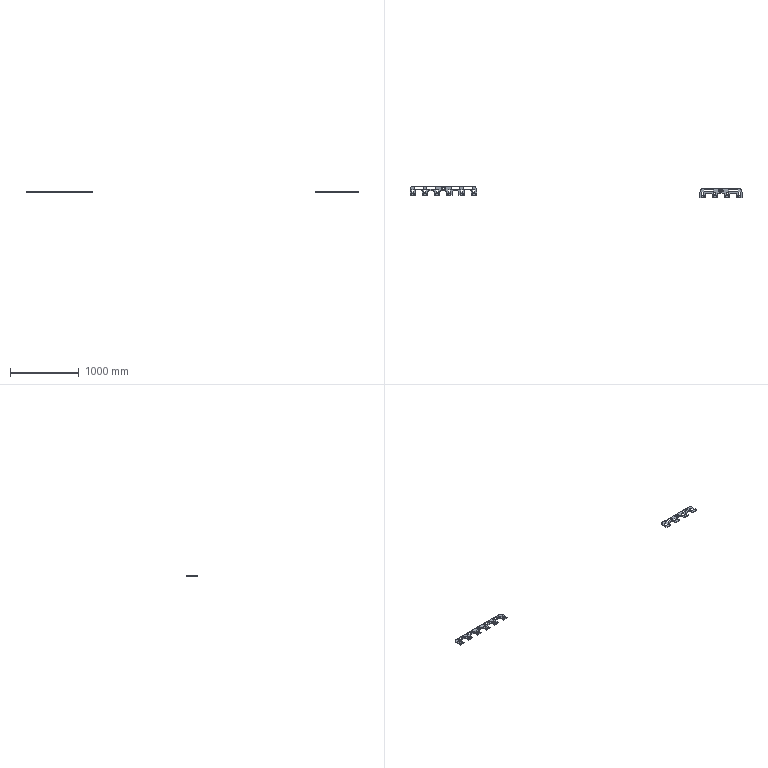NC program | NX | posted with a generic post | part box 4825 x 168.213 x 13 mm
Lines 124 to 1113 of 9095:
(ZLEVEL_PROFILE , TOOL : D10)
N228 T10 M6
N230 G54
N232 G17 G0 G90 X-46.824 Y72.1 S9500 M3
N234 G43 Z30. H10
N236 Z1.5
N238 G94 G1 X-0.002 Z-0.954 F1000.
N240 X255.6 F3500.
N242 G2 X310.7 Y16.999 R55.1
N244 G1 Y-67.
N246 G2 X305.6 Y-72.1 R5.1
N248 G1 X227.8
N250 G2 X222.7 Y-67. R5.1
N252 G1 Y-20.95
N254 G3 X207.8 Y-6.05 R14.9
N256 G1 X147.8
N258 G3 X132.9 Y-20.95 R14.9
N260 G1 Y-67.
N262 G2 X127.8 Y-72.1 R5.1
N264 G1 X50.
N266 G2 X44.9 Y-67. R5.1
N268 G1 Y-20.95
N270 G3 X30. Y-6.05 R14.9
N272 G1 X-30.
N274 G3 X-44.9 Y-20.95 R14.9
N276 G1 Y-67.
N278 G2 X-50. Y-72.1 R5.1
N280 G1 X-127.8
N282 G2 X-132.9 Y-67. R5.1
N284 G1 Y-20.95
N286 G3 X-147.8 Y-6.05 R14.9
N288 G1 X-207.804
N290 G3 X-222.7 Y-20.95 R14.9
N292 G1 Y-67.
N294 G2 X-227.8 Y-72.1 R5.1
N296 G1 X-305.6
N298 G2 X-310.7 Y-67. R5.1
N300 G1 Y16.999
N302 G2 X-255.604 Y72.1 R55.1
N304 G1 X-0.002
N306 X54.644 Z-1.908
N308 X255.6
N310 G2 X310.7 Y16.999 R55.1
N312 G1 Y-67.
N314 G2 X305.6 Y-72.1 R5.1
N316 G1 X227.8
N318 G2 X222.7 Y-67. R5.1
N320 G1 Y-20.95
N322 G3 X207.8 Y-6.05 R14.9
N324 G1 X147.8
N326 G3 X132.9 Y-20.95 R14.9
N328 G1 Y-67.
N330 G2 X127.8 Y-72.1 R5.1
N332 G1 X50.
N334 G2 X44.9 Y-67. R5.1
N336 G1 Y-20.95
N338 G3 X30. Y-6.05 R14.9
N340 G1 X-30.
N342 G3 X-44.9 Y-20.95 R14.9
N344 G1 Y-67.
N346 G2 X-50. Y-72.1 R5.1
N348 G1 X-127.8
N350 G2 X-132.9 Y-67. R5.1
N352 G1 Y-20.95
N354 G3 X-147.8 Y-6.05 R14.9
N356 G1 X-207.804
N358 G3 X-222.7 Y-20.95 R14.9
N360 G1 Y-67.
N362 G2 X-227.8 Y-72.1 R5.1
N364 G1 X-305.6
N366 G2 X-310.7 Y-67. R5.1
N368 G1 Y16.999
N370 G2 X-255.604 Y72.1 R55.1
N372 G1 X-0.002
N374 X54.644 Z-2.862
N376 X255.6
N378 G2 X310.7 Y16.999 R55.1
N380 G1 Y-67.
N382 G2 X305.6 Y-72.1 R5.1
N384 G1 X227.8
N386 G2 X222.7 Y-67. R5.1
N388 G1 Y-20.95
N390 G3 X207.8 Y-6.05 R14.9
N392 G1 X147.8
N394 G3 X132.9 Y-20.95 R14.9
N396 G1 Y-67.
N398 G2 X127.8 Y-72.1 R5.1
N400 G1 X50.
N402 G2 X44.9 Y-67. R5.1
N404 G1 Y-20.95
N406 G3 X30. Y-6.05 R14.9
N408 G1 X-30.
N410 G3 X-44.9 Y-20.95 R14.9
N412 G1 Y-67.
N414 G2 X-50. Y-72.1 R5.1
N416 G1 X-127.8
N418 G2 X-132.9 Y-67. R5.1
N420 G1 Y-20.95
N422 G3 X-147.8 Y-6.05 R14.9
N424 G1 X-207.804
N426 G3 X-222.7 Y-20.95 R14.9
N428 G1 Y-67.
N430 G2 X-227.8 Y-72.1 R5.1
N432 G1 X-305.6
N434 G2 X-310.7 Y-67. R5.1
N436 G1 Y16.999
N438 G2 X-255.604 Y72.1 R55.1
N440 G1 X-0.002
N442 X54.644 Z-3.815
N444 X255.6
N446 G2 X310.7 Y16.999 R55.1
N448 G1 Y-67.
N450 G2 X305.6 Y-72.1 R5.1
N452 G1 X227.8
N454 G2 X222.7 Y-67. R5.1
N456 G1 Y-20.95
N458 G3 X207.8 Y-6.05 R14.9
N460 G1 X147.8
N462 G3 X132.9 Y-20.95 R14.9
N464 G1 Y-67.
N466 G2 X127.8 Y-72.1 R5.1
N468 G1 X50.
N470 G2 X44.9 Y-67. R5.1
N472 G1 Y-20.95
N474 G3 X30. Y-6.05 R14.9
N476 G1 X-30.
N478 G3 X-44.9 Y-20.95 R14.9
N480 G1 Y-67.
N482 G2 X-50. Y-72.1 R5.1
N484 G1 X-127.8
N486 G2 X-132.9 Y-67. R5.1
N488 G1 Y-20.95
N490 G3 X-147.8 Y-6.05 R14.9
N492 G1 X-207.804
N494 G3 X-222.7 Y-20.95 R14.9
N496 G1 Y-67.
N498 G2 X-227.8 Y-72.1 R5.1
N500 G1 X-305.6
N502 G2 X-310.7 Y-67. R5.1
N504 G1 Y16.999
N506 G2 X-255.604 Y72.1 R55.1
N508 G1 X-0.002
N510 X54.644 Z-4.769
N512 X255.6
N514 G2 X310.7 Y16.999 R55.1
N516 G1 Y-67.
N518 G2 X305.6 Y-72.1 R5.1
N520 G1 X227.8
N522 G2 X222.7 Y-67. R5.1
N524 G1 Y-20.95
N526 G3 X207.8 Y-6.05 R14.9
N528 G1 X147.8
N530 G3 X132.9 Y-20.95 R14.9
N532 G1 Y-67.
N534 G2 X127.8 Y-72.1 R5.1
N536 G1 X50.
N538 G2 X44.9 Y-67. R5.1
N540 G1 Y-20.95
N542 G3 X30. Y-6.05 R14.9
N544 G1 X-30.
N546 G3 X-44.9 Y-20.95 R14.9
N548 G1 Y-67.
N550 G2 X-50. Y-72.1 R5.1
N552 G1 X-127.8
N554 G2 X-132.9 Y-67. R5.1
N556 G1 Y-20.95
N558 G3 X-147.8 Y-6.05 R14.9
N560 G1 X-207.804
N562 G3 X-222.7 Y-20.95 R14.9
N564 G1 Y-67.
N566 G2 X-227.8 Y-72.1 R5.1
N568 G1 X-305.6
N570 G2 X-310.7 Y-67. R5.1
N572 G1 Y16.999
N574 G2 X-255.604 Y72.1 R55.1
N576 G1 X-0.002
N578 X54.644 Z-5.723
N580 X255.6
N582 G2 X310.7 Y16.999 R55.1
N584 G1 Y-67.
N586 G2 X305.6 Y-72.1 R5.1
N588 G1 X227.8
N590 G2 X222.7 Y-67. R5.1
N592 G1 Y-20.95
N594 G3 X207.8 Y-6.05 R14.9
N596 G1 X147.8
N598 G3 X132.9 Y-20.95 R14.9
N600 G1 Y-67.
N602 G2 X127.8 Y-72.1 R5.1
N604 G1 X50.
N606 G2 X44.9 Y-67. R5.1
N608 G1 Y-20.95
N610 G3 X30. Y-6.05 R14.9
N612 G1 X-30.
N614 G3 X-44.9 Y-20.95 R14.9
N616 G1 Y-67.
N618 G2 X-50. Y-72.1 R5.1
N620 G1 X-127.8
N622 G2 X-132.9 Y-67. R5.1
N624 G1 Y-20.95
N626 G3 X-147.8 Y-6.05 R14.9
N628 G1 X-207.804
N630 G3 X-222.7 Y-20.95 R14.9
N632 G1 Y-67.
N634 G2 X-227.8 Y-72.1 R5.1
N636 G1 X-305.6
N638 G2 X-310.7 Y-67. R5.1
N640 G1 Y16.999
N642 G2 X-255.604 Y72.1 R55.1
N644 G1 X-0.002
N646 X54.644 Z-6.677
N648 X255.6
N650 G2 X310.7 Y16.999 R55.1
N652 G1 Y-67.
N654 G2 X305.6 Y-72.1 R5.1
N656 G1 X227.8
N658 G2 X222.7 Y-67. R5.1
N660 G1 Y-20.95
N662 G3 X207.8 Y-6.05 R14.9
N664 G1 X147.8
N666 G3 X132.9 Y-20.95 R14.9
N668 G1 Y-67.
N670 G2 X127.8 Y-72.1 R5.1
N672 G1 X50.
N674 G2 X44.9 Y-67. R5.1
N676 G1 Y-20.95
N678 G3 X30. Y-6.05 R14.9
N680 G1 X-30.
N682 G3 X-44.9 Y-20.95 R14.9
N684 G1 Y-67.
N686 G2 X-50. Y-72.1 R5.1
N688 G1 X-127.8
N690 G2 X-132.9 Y-67. R5.1
N692 G1 Y-20.95
N694 G3 X-147.8 Y-6.05 R14.9
N696 G1 X-207.804
N698 G3 X-222.7 Y-20.95 R14.9
N700 G1 Y-67.
N702 G2 X-227.8 Y-72.1 R5.1
N704 G1 X-305.6
N706 G2 X-310.7 Y-67. R5.1
N708 G1 Y16.999
N710 G2 X-255.604 Y72.1 R55.1
N712 G1 X-0.002
N714 X54.644 Z-7.631
N716 X255.6
N718 G2 X310.7 Y16.999 R55.1
N720 G1 Y-67.
N722 G2 X305.6 Y-72.1 R5.1
N724 G1 X227.8
N726 G2 X222.7 Y-67. R5.1
N728 G1 Y-20.95
N730 G3 X207.8 Y-6.05 R14.9
N732 G1 X147.8
N734 G3 X132.9 Y-20.95 R14.9
N736 G1 Y-67.
N738 G2 X127.8 Y-72.1 R5.1
N740 G1 X50.
N742 G2 X44.9 Y-67. R5.1
N744 G1 Y-20.95
N746 G3 X30. Y-6.05 R14.9
N748 G1 X-30.
N750 G3 X-44.9 Y-20.95 R14.9
N752 G1 Y-67.
N754 G2 X-50. Y-72.1 R5.1
N756 G1 X-127.8
N758 G2 X-132.9 Y-67. R5.1
N760 G1 Y-20.95
N762 G3 X-147.8 Y-6.05 R14.9
N764 G1 X-207.804
N766 G3 X-222.7 Y-20.95 R14.9
N768 G1 Y-67.
N770 G2 X-227.8 Y-72.1 R5.1
N772 G1 X-305.6
N774 G2 X-310.7 Y-67. R5.1
N776 G1 Y16.999
N778 G2 X-255.604 Y72.1 R55.1
N780 G1 X-0.002
N782 X54.644 Z-8.585
N784 X255.6
N786 G2 X310.7 Y16.999 R55.1
N788 G1 Y-67.
N790 G2 X305.6 Y-72.1 R5.1
N792 G1 X227.8
N794 G2 X222.7 Y-67. R5.1
N796 G1 Y-20.95
N798 G3 X207.8 Y-6.05 R14.9
N800 G1 X147.8
N802 G3 X132.9 Y-20.95 R14.9
N804 G1 Y-67.
N806 G2 X127.8 Y-72.1 R5.1
N808 G1 X50.
N810 G2 X44.9 Y-67. R5.1
N812 G1 Y-20.95
N814 G3 X30. Y-6.05 R14.9
N816 G1 X-30.
N818 G3 X-44.9 Y-20.95 R14.9
N820 G1 Y-67.
N822 G2 X-50. Y-72.1 R5.1
N824 G1 X-127.8
N826 G2 X-132.9 Y-67. R5.1
N828 G1 Y-20.95
N830 G3 X-147.8 Y-6.05 R14.9
N832 G1 X-207.804
N834 G3 X-222.7 Y-20.95 R14.9
N836 G1 Y-67.
N838 G2 X-227.8 Y-72.1 R5.1
N840 G1 X-305.6
N842 G2 X-310.7 Y-67. R5.1
N844 G1 Y16.999
N846 G2 X-255.604 Y72.1 R55.1
N848 G1 X-0.002
N850 X54.644 Z-9.538
N852 X255.6
N854 G2 X310.7 Y16.999 R55.1
N856 G1 Y-67.
N858 G2 X305.6 Y-72.1 R5.1
N860 G1 X227.8
N862 G2 X222.7 Y-67. R5.1
N864 G1 Y-20.95
N866 G3 X207.8 Y-6.05 R14.9
N868 G1 X147.8
N870 G3 X132.9 Y-20.95 R14.9
N872 G1 Y-67.
N874 G2 X127.8 Y-72.1 R5.1
N876 G1 X50.
N878 G2 X44.9 Y-67. R5.1
N880 G1 Y-20.95
N882 G3 X30. Y-6.05 R14.9
N884 G1 X-30.
N886 G3 X-44.9 Y-20.95 R14.9
N888 G1 Y-67.
N890 G2 X-50. Y-72.1 R5.1
N892 G1 X-127.8
N894 G2 X-132.9 Y-67. R5.1
N896 G1 Y-20.95
N898 G3 X-147.8 Y-6.05 R14.9
N900 G1 X-207.804
N902 G3 X-222.7 Y-20.95 R14.9
N904 G1 Y-67.
N906 G2 X-227.8 Y-72.1 R5.1
N908 G1 X-305.6
N910 G2 X-310.7 Y-67. R5.1
N912 G1 Y16.999
N914 G2 X-255.604 Y72.1 R55.1
N916 G1 X-0.002
N918 X54.644 Z-10.492
N920 X255.6
N922 G2 X310.7 Y16.999 R55.1
N924 G1 Y-67.
N926 G2 X305.6 Y-72.1 R5.1
N928 G1 X227.8
N930 G2 X222.7 Y-67. R5.1
N932 G1 Y-20.95
N934 G3 X207.8 Y-6.05 R14.9
N936 G1 X147.8
N938 G3 X132.9 Y-20.95 R14.9
N940 G1 Y-67.
N942 G2 X127.8 Y-72.1 R5.1
N944 G1 X50.
N946 G2 X44.9 Y-67. R5.1
N948 G1 Y-20.95
N950 G3 X30. Y-6.05 R14.9
N952 G1 X-30.
N954 G3 X-44.9 Y-20.95 R14.9
N956 G1 Y-67.
N958 G2 X-50. Y-72.1 R5.1
N960 G1 X-127.8
N962 G2 X-132.9 Y-67. R5.1
N964 G1 Y-20.95
N966 G3 X-147.8 Y-6.05 R14.9
N968 G1 X-207.804
N970 G3 X-222.7 Y-20.95 R14.9
N972 G1 Y-67.
N974 G2 X-227.8 Y-72.1 R5.1
N976 G1 X-305.6
N978 G2 X-310.7 Y-67. R5.1
N980 G1 Y16.999
N982 G2 X-255.604 Y72.1 R55.1
N984 G1 X-0.002
N986 X54.644 Z-11.446
N988 X255.6
N990 G2 X310.7 Y16.999 R55.1
N992 G1 Y-67.
N994 G2 X305.6 Y-72.1 R5.1
N996 G1 X227.8
N998 G2 X222.7 Y-67. R5.1
N1000 G1 Y-20.95
N1002 G3 X207.8 Y-6.05 R14.9
N1004 G1 X147.8
N1006 G3 X132.9 Y-20.95 R14.9
N1008 G1 Y-67.
N1010 G2 X127.8 Y-72.1 R5.1
N1012 G1 X50.
N1014 G2 X44.9 Y-67. R5.1
N1016 G1 Y-20.95
N1018 G3 X30. Y-6.05 R14.9
N1020 G1 X-30.
N1022 G3 X-44.9 Y-20.95 R14.9
N1024 G1 Y-67.
N1026 G2 X-50. Y-72.1 R5.1
N1028 G1 X-127.8
N1030 G2 X-132.9 Y-67. R5.1
N1032 G1 Y-20.95
N1034 G3 X-147.8 Y-6.05 R14.9
N1036 G1 X-207.804
N1038 G3 X-222.7 Y-20.95 R14.9
N1040 G1 Y-67.
N1042 G2 X-227.8 Y-72.1 R5.1
N1044 G1 X-305.6
N1046 G2 X-310.7 Y-67. R5.1
N1048 G1 Y16.999
N1050 G2 X-255.604 Y72.1 R55.1
N1052 G1 X-0.002
N1054 X54.644 Z-12.4
N1056 X255.6
N1058 G2 X310.7 Y16.999 R55.1
N1060 G1 Y-67.
N1062 G2 X305.6 Y-72.1 R5.1
N1064 G1 X227.8
N1066 G2 X222.7 Y-67. R5.1
N1068 G1 Y-20.95
N1070 G3 X207.8 Y-6.05 R14.9
N1072 G1 X147.8
N1074 G3 X132.9 Y-20.95 R14.9
N1076 G1 Y-67.
N1078 G2 X127.8 Y-72.1 R5.1
N1080 G1 X50.
N1082 G2 X44.9 Y-67. R5.1
N1084 G1 Y-20.95
N1086 G3 X30. Y-6.05 R14.9
N1088 G1 X-30.
N1090 G3 X-44.9 Y-20.95 R14.9
N1092 G1 Y-67.
N1094 G2 X-50. Y-72.1 R5.1
N1096 G1 X-127.8
N1098 G2 X-132.9 Y-67. R5.1
N1100 G1 Y-20.95
N1102 G3 X-147.8 Y-6.05 R14.9
N1104 G1 X-207.804
N1106 G3 X-222.7 Y-20.95 R14.9
N1108 G1 Y-67.
N1110 G2 X-227.8 Y-72.1 R5.1
N1112 G1 X-305.6
N1114 G2 X-310.7 Y-67. R5.1
N1116 G1 Y16.999
N1118 G2 X-255.604 Y72.1 R55.1
N1120 G1 X54.644
N1122 Z-10.9
N1124 G0 Z30.
(ZLEVEL_PROFILE_COPY_2 , TOOL : D10)
N1126 X-130.244 Y51.9
N1128 Z1.5
N1130 G1 X-177.8 Z-0.992 F1000.
N1132 X-236.6 F3500.
N1134 Y30.1
N1136 X-119.
N1138 Y51.9
N1140 X-177.8
N1142 X-234.649 Z-1.985
N1144 X-236.6
N1146 Y30.1
N1148 X-119.
N1150 Y51.9
N1152 X-177.8
N1154 X-234.649 Z-2.977
N1156 X-236.6
N1158 Y30.1
N1160 X-119.
N1162 Y51.9
N1164 X-177.8
N1166 X-234.649 Z-3.969
N1168 X-236.6
N1170 Y30.1
N1172 X-119.
N1174 Y51.9
N1176 X-177.8
N1178 X-234.649 Z-4.962
N1180 X-236.6
N1182 Y30.1
N1184 X-119.
N1186 Y51.9
N1188 X-177.8
N1190 X-234.649 Z-5.954
N1192 X-236.6
N1194 Y30.1
N1196 X-119.
N1198 Y51.9
N1200 X-177.8
N1202 X-234.649 Z-6.946
N1204 X-236.6
N1206 Y30.1
N1208 X-119.
N1210 Y51.9
N1212 X-177.8
N1214 X-234.649 Z-7.938
N1216 X-236.6
N1218 Y30.1
N1220 X-119.
N1222 Y51.9
N1224 X-177.8
N1226 X-234.649 Z-8.931
N1228 X-236.6
N1230 Y30.1
N1232 X-119.
N1234 Y51.9
N1236 X-177.8
N1238 X-234.649 Z-9.923
N1240 X-236.6
N1242 Y30.1
N1244 X-119.
N1246 Y51.9
N1248 X-177.8
N1250 X-234.649 Z-10.915
N1252 X-236.6
N1254 Y30.1
N1256 X-119.
N1258 Y51.9
N1260 X-177.8
N1262 X-234.649 Z-11.908
N1264 X-236.6
N1266 Y30.1
N1268 X-119.
N1270 Y51.9
N1272 X-177.8
N1274 X-234.649 Z-12.9
N1276 X-236.6
N1278 Y30.1
N1280 X-119.
N1282 Y51.9
N1284 X-234.649
N1286 Z-11.4
N1288 G0 Z30.
N1290 X-9.861 Y33.882
N1292 Z1.5
N1294 G1 X-9.909 Y32.876 Z1.447 F1000.
N1296 X-9.822 Y31.684 Z1.385
N1298 X-9.593 Y30.512 Z1.322
N1300 X-9.223 Y29.375 Z1.259
N1302 X-8.72 Y28.291 Z1.197
N1304 X-8.262 Y27.528 Z1.15
N1306 X-7.548 Y26.579 Z1.088
N1308 X-6.726 Y25.722 Z1.026
N1310 X-5.808 Y24.97 Z0.963
N1312 X-4.805 Y24.333 Z0.901
N1314 X-3.734 Y23.821 Z0.839
N1316 X-2.61 Y23.44 Z0.777
N1318 X-1.447 Y23.196 Z0.714
N1320 X-0.265 Y23.094 Z0.652
N1322 X0.922 Y23.133 Z0.59
N1324 X2.096 Y23.314 Z0.528
N1326 X3.239 Y23.634 Z0.466
N1328 X4.336 Y24.089 Z0.403
N1330 X5.371 Y24.672 Z0.341
N1332 X6.328 Y25.374 Z0.279
N1334 X7.195 Y26.185 Z0.217
N1336 X7.958 Y27.095 Z0.154
N1338 X8.456 Y27.833 Z0.108
N1340 X9.026 Y28.909 Z0.044
N1342 X9.46 Y30.047 Z-0.02
N1344 X9.751 Y31.23 Z-0.084
N1346 X9.894 Y32.439 Z-0.148
N1348 X9.888 Y33.657 Z-0.211
N1350 X9.733 Y34.865 Z-0.275
N1352 X9.431 Y36.045 Z-0.339
N1354 X8.986 Y37.179 Z-0.403
N1356 X8.406 Y38.249 Z-0.467
N1358 X7.698 Y39.241 Z-0.531
N1360 X6.874 Y40.138 Z-0.594
N1362 X5.947 Y40.927 Z-0.658
N1364 X4.93 Y41.597 Z-0.722
N1366 X3.838 Y42.137 Z-0.786
N1368 X2.688 Y42.538 Z-0.85
N1370 X1.821 Y42.741 Z-0.896
N1372 X1.136 Y42.845 Z-0.933
N1374 X0.445 Y42.9 Z-0.969
N1376 X0. Z-0.992
N1378 G3 X-9.9 Y33. R9.9 F3500.
N1380 X0. Y42.9 R-9.9
N1382 G1 X-0.222 Y42.898 Z-0.997
N1384 X-0.444 Y42.89 Z-1.002
N1386 X-0.666 Y42.878 Z-1.006
N1388 X-0.887 Y42.86 Z-1.011
N1390 X-1.108 Y42.838 Z-1.016
N1392 X-1.329 Y42.81 Z-1.021
N1394 X-1.549 Y42.778 Z-1.025
N1396 X-1.768 Y42.741 Z-1.03
N1398 X-1.986 Y42.699 Z-1.035
N1400 X-2.203 Y42.652 Z-1.04
N1402 X-2.419 Y42.6 Z-1.044
N1404 X-2.634 Y42.543 Z-1.049
N1406 X-2.847 Y42.482 Z-1.054
N1408 X-3.059 Y42.415 Z-1.058
N1410 X-3.27 Y42.344 Z-1.063
N1412 X-3.479 Y42.269 Z-1.068
N1414 X-3.686 Y42.188 Z-1.073
N1416 X-3.891 Y42.103 Z-1.077
N1418 X-4.094 Y42.014 Z-1.082
N1420 X-4.295 Y41.92 Z-1.087
N1422 X-4.495 Y41.821 Z-1.092
N1424 X-4.691 Y41.718 Z-1.096
N1426 X-4.886 Y41.61 Z-1.101
N1428 X-5.078 Y41.499 Z-1.106
N1430 X-5.267 Y41.383 Z-1.11
N1432 X-5.454 Y41.262 Z-1.115
N1434 X-5.638 Y41.138 Z-1.12
N1436 X-5.819 Y41.009 Z-1.125
N1438 X-5.997 Y40.877 Z-1.129
N1440 X-6.173 Y40.74 Z-1.134
N1442 X-6.345 Y40.6 Z-1.139
N1444 X-6.514 Y40.455 Z-1.144
N1446 X-6.679 Y40.307 Z-1.148
N1448 X-6.842 Y40.156 Z-1.153
N1450 X-7. Y40. Z-1.158
N1452 X-7.156 Y39.842 Z-1.162
N1454 X-7.307 Y39.679 Z-1.167
N1456 X-7.455 Y39.514 Z-1.172
N1458 X-7.6 Y39.345 Z-1.177
N1460 X-7.74 Y39.173 Z-1.181
N1462 X-7.877 Y38.997 Z-1.186
N1464 X-8.009 Y38.819 Z-1.191
N1466 X-8.138 Y38.638 Z-1.195
N1468 X-8.262 Y38.454 Z-1.2
N1470 X-8.383 Y38.267 Z-1.205
N1472 X-8.499 Y38.078 Z-1.21
N1474 X-8.61 Y37.886 Z-1.214
N1476 X-8.718 Y37.691 Z-1.219
N1478 X-8.821 Y37.495 Z-1.224
N1480 X-8.92 Y37.295 Z-1.229
N1482 X-9.014 Y37.094 Z-1.233
N1484 X-9.103 Y36.891 Z-1.238
N1486 X-9.188 Y36.686 Z-1.243
N1488 X-9.269 Y36.479 Z-1.247
N1490 X-9.344 Y36.27 Z-1.252
N1492 X-9.415 Y36.059 Z-1.257
N1494 X-9.482 Y35.847 Z-1.262
N1496 X-9.543 Y35.634 Z-1.266
N1498 X-9.6 Y35.419 Z-1.271
N1500 X-9.652 Y35.203 Z-1.276
N1502 X-9.699 Y34.986 Z-1.281
N1504 X-9.741 Y34.768 Z-1.285
N1506 X-9.778 Y34.549 Z-1.29
N1508 X-9.81 Y34.329 Z-1.295
N1510 X-9.838 Y34.108 Z-1.299
N1512 X-9.86 Y33.887 Z-1.304
N1514 X-9.878 Y33.666 Z-1.309
N1516 X-9.89 Y33.444 Z-1.314
N1518 X-9.898 Y33.222 Z-1.318
N1520 X-9.9 Y33. Z-1.323
N1522 X-9.898 Y32.778 Z-1.328
N1524 X-9.89 Y32.556 Z-1.333
N1526 X-9.878 Y32.334 Z-1.337
N1528 X-9.86 Y32.113 Z-1.342
N1530 X-9.838 Y31.892 Z-1.347
N1532 X-9.81 Y31.671 Z-1.351
N1534 X-9.778 Y31.451 Z-1.356
N1536 X-9.741 Y31.232 Z-1.361
N1538 X-9.699 Y31.014 Z-1.366
N1540 X-9.652 Y30.797 Z-1.37
N1542 X-9.6 Y30.581 Z-1.375
N1544 X-9.543 Y30.366 Z-1.38
N1546 X-9.482 Y30.153 Z-1.385
N1548 X-9.415 Y29.941 Z-1.389
N1550 X-9.344 Y29.73 Z-1.394
N1552 X-9.269 Y29.521 Z-1.399
N1554 X-9.188 Y29.314 Z-1.403
N1556 X-9.103 Y29.109 Z-1.408
N1558 X-9.014 Y28.906 Z-1.413
N1560 X-8.92 Y28.705 Z-1.418
N1562 X-8.821 Y28.505 Z-1.422
N1564 X-8.718 Y28.309 Z-1.427
N1566 X-8.61 Y28.114 Z-1.432
N1568 X-8.499 Y27.922 Z-1.436
N1570 X-8.383 Y27.733 Z-1.441
N1572 X-8.262 Y27.546 Z-1.446
N1574 X-8.138 Y27.362 Z-1.451
N1576 X-8.009 Y27.181 Z-1.455
N1578 X-7.877 Y27.003 Z-1.46
N1580 X-7.74 Y26.827 Z-1.465
N1582 X-7.6 Y26.655 Z-1.47
N1584 X-7.455 Y26.486 Z-1.474
N1586 X-7.307 Y26.321 Z-1.479
N1588 X-7.156 Y26.158 Z-1.484
N1590 X-7. Y26. Z-1.488
N1592 X-6.842 Y25.844 Z-1.493
N1594 X-6.679 Y25.693 Z-1.498
N1596 X-6.514 Y25.545 Z-1.503
N1598 X-6.345 Y25.4 Z-1.507
N1600 X-6.173 Y25.26 Z-1.512
N1602 X-5.997 Y25.123 Z-1.517
N1604 X-5.819 Y24.991 Z-1.522
N1606 X-5.638 Y24.862 Z-1.526
N1608 X-5.454 Y24.738 Z-1.531
N1610 X-5.267 Y24.617 Z-1.536
N1612 X-5.078 Y24.501 Z-1.54
N1614 X-4.886 Y24.39 Z-1.545
N1616 X-4.691 Y24.282 Z-1.55
N1618 X-4.495 Y24.179 Z-1.555
N1620 X-4.295 Y24.08 Z-1.559
N1622 X-4.094 Y23.986 Z-1.564
N1624 X-3.891 Y23.897 Z-1.569
N1626 X-3.686 Y23.812 Z-1.574
N1628 X-3.479 Y23.731 Z-1.578
N1630 X-3.27 Y23.656 Z-1.583
N1632 X-3.059 Y23.585 Z-1.588
N1634 X-2.847 Y23.518 Z-1.592
N1636 X-2.634 Y23.457 Z-1.597
N1638 X-2.419 Y23.4 Z-1.602
N1640 X-2.203 Y23.348 Z-1.607
N1642 X-1.986 Y23.301 Z-1.611
N1644 X-1.768 Y23.259 Z-1.616
N1646 X-1.549 Y23.222 Z-1.621
N1648 X-1.329 Y23.19 Z-1.625
N1650 X-1.108 Y23.162 Z-1.63
N1652 X-0.887 Y23.14 Z-1.635
N1654 X-0.666 Y23.122 Z-1.64
N1656 X-0.444 Y23.11 Z-1.644
N1658 X-0.222 Y23.102 Z-1.649
N1660 X0. Y23.1 Z-1.654
N1662 X0.222 Y23.102 Z-1.659
N1664 X0.444 Y23.11 Z-1.663
N1666 X0.666 Y23.122 Z-1.668
N1668 X0.887 Y23.14 Z-1.673
N1670 X1.108 Y23.162 Z-1.677
N1672 X1.329 Y23.19 Z-1.682
N1674 X1.549 Y23.222 Z-1.687
N1676 X1.768 Y23.259 Z-1.692
N1678 X1.986 Y23.301 Z-1.696
N1680 X2.203 Y23.348 Z-1.701
N1682 X2.419 Y23.4 Z-1.706
N1684 X2.634 Y23.457 Z-1.711
N1686 X2.847 Y23.518 Z-1.715
N1688 X3.059 Y23.585 Z-1.72
N1690 X3.27 Y23.656 Z-1.725
N1692 X3.479 Y23.731 Z-1.729
N1694 X3.686 Y23.812 Z-1.734
N1696 X3.891 Y23.897 Z-1.739
N1698 X4.094 Y23.986 Z-1.744
N1700 X4.295 Y24.08 Z-1.748
N1702 X4.495 Y24.179 Z-1.753
N1704 X4.691 Y24.282 Z-1.758
N1706 X4.886 Y24.39 Z-1.763
N1708 X5.078 Y24.501 Z-1.767
N1710 X5.267 Y24.617 Z-1.772
N1712 X5.454 Y24.738 Z-1.777
N1714 X5.638 Y24.862 Z-1.781
N1716 X5.819 Y24.991 Z-1.786
N1718 X5.997 Y25.123 Z-1.791
N1720 X6.173 Y25.26 Z-1.796
N1722 X6.345 Y25.4 Z-1.8
N1724 X6.514 Y25.545 Z-1.805
N1726 X6.679 Y25.693 Z-1.81
N1728 X6.842 Y25.844 Z-1.815
N1730 X7. Y26. Z-1.819
N1732 X7.156 Y26.158 Z-1.824
N1734 X7.307 Y26.321 Z-1.829
N1736 X7.455 Y26.486 Z-1.833
N1738 X7.6 Y26.655 Z-1.838
N1740 X7.74 Y26.827 Z-1.843
N1742 X7.877 Y27.003 Z-1.848
N1744 X8.009 Y27.181 Z-1.852
N1746 X8.138 Y27.362 Z-1.857
N1748 X8.262 Y27.546 Z-1.862
N1750 X8.383 Y27.733 Z-1.866
N1752 X8.499 Y27.922 Z-1.871
N1754 X8.61 Y28.114 Z-1.876
N1756 X8.718 Y28.309 Z-1.881
N1758 X8.821 Y28.505 Z-1.885
N1760 X8.92 Y28.705 Z-1.89
N1762 X9.014 Y28.906 Z-1.895
N1764 X9.103 Y29.109 Z-1.9
N1766 X9.188 Y29.314 Z-1.904
N1768 X9.269 Y29.521 Z-1.909
N1770 X9.344 Y29.73 Z-1.914
N1772 X9.415 Y29.941 Z-1.918
N1774 X9.482 Y30.153 Z-1.923
N1776 X9.543 Y30.366 Z-1.928
N1778 X9.6 Y30.581 Z-1.933
N1780 X9.652 Y30.797 Z-1.937
N1782 X9.699 Y31.014 Z-1.942
N1784 X9.741 Y31.232 Z-1.947
N1786 X9.778 Y31.451 Z-1.952
N1788 X9.81 Y31.671 Z-1.956
N1790 X9.838 Y31.892 Z-1.961
N1792 X9.86 Y32.113 Z-1.966
N1794 X9.878 Y32.334 Z-1.97
N1796 X9.89 Y32.556 Z-1.975
N1798 X9.898 Y32.778 Z-1.98
N1800 X9.9 Y33. Z-1.985
N1802 G3 X0. Y42.9 R9.9
N1804 G1 X-0.222 Y42.898 Z-1.989
N1806 X-0.444 Y42.89 Z-1.994
N1808 X-0.666 Y42.878 Z-1.999
N1810 X-0.887 Y42.86 Z-2.004
N1812 X-1.108 Y42.838 Z-2.008
N1814 X-1.329 Y42.81 Z-2.013
N1816 X-1.549 Y42.778 Z-2.018
N1818 X-1.768 Y42.741 Z-2.022
N1820 X-1.986 Y42.699 Z-2.027
N1822 X-2.203 Y42.652 Z-2.032
N1824 X-2.419 Y42.6 Z-2.037
N1826 X-2.634 Y42.543 Z-2.041
N1828 X-2.847 Y42.482 Z-2.046
N1830 X-3.059 Y42.415 Z-2.051
N1832 X-3.27 Y42.344 Z-2.055
N1834 X-3.479 Y42.269 Z-2.06
N1836 X-3.686 Y42.188 Z-2.065
N1838 X-3.891 Y42.103 Z-2.07
N1840 X-4.094 Y42.014 Z-2.074
N1842 X-4.295 Y41.92 Z-2.079
N1844 X-4.495 Y41.821 Z-2.084
N1846 X-4.691 Y41.718 Z-2.089
N1848 X-4.886 Y41.61 Z-2.093
N1850 X-5.078 Y41.499 Z-2.098
N1852 X-5.267 Y41.383 Z-2.103
N1854 X-5.454 Y41.262 Z-2.107
N1856 X-5.638 Y41.138 Z-2.112
N1858 X-5.819 Y41.009 Z-2.117
N1860 X-5.997 Y40.877 Z-2.122
N1862 X-6.173 Y40.74 Z-2.126
N1864 X-6.345 Y40.6 Z-2.131
N1866 X-6.514 Y40.455 Z-2.136
N1868 X-6.679 Y40.307 Z-2.141
N1870 X-6.842 Y40.156 Z-2.145
N1872 X-7. Y40. Z-2.15
N1874 X-7.156 Y39.842 Z-2.155
N1876 X-7.307 Y39.679 Z-2.159
N1878 X-7.455 Y39.514 Z-2.164
N1880 X-7.6 Y39.345 Z-2.169
N1882 X-7.74 Y39.173 Z-2.174
N1884 X-7.877 Y38.997 Z-2.178
N1886 X-8.009 Y38.819 Z-2.183
N1888 X-8.138 Y38.638 Z-2.188
N1890 X-8.262 Y38.454 Z-2.193
N1892 X-8.383 Y38.267 Z-2.197
N1894 X-8.499 Y38.078 Z-2.202
N1896 X-8.61 Y37.886 Z-2.207
N1898 X-8.718 Y37.691 Z-2.211
N1900 X-8.821 Y37.495 Z-2.216
N1902 X-8.92 Y37.295 Z-2.221
N1904 X-9.014 Y37.094 Z-2.226
N1906 X-9.103 Y36.891 Z-2.23
N1908 X-9.188 Y36.686 Z-2.235
N1910 X-9.269 Y36.479 Z-2.24
N1912 X-9.344 Y36.27 Z-2.245
N1914 X-9.415 Y36.059 Z-2.249
N1916 X-9.482 Y35.847 Z-2.254
N1918 X-9.543 Y35.634 Z-2.259
N1920 X-9.6 Y35.419 Z-2.263
N1922 X-9.652 Y35.203 Z-2.268
N1924 X-9.699 Y34.986 Z-2.273
N1926 X-9.741 Y34.768 Z-2.278
N1928 X-9.778 Y34.549 Z-2.282
N1930 X-9.81 Y34.329 Z-2.287
N1932 X-9.838 Y34.108 Z-2.292
N1934 X-9.86 Y33.887 Z-2.296
N1936 X-9.878 Y33.666 Z-2.301
N1938 X-9.89 Y33.444 Z-2.306
N1940 X-9.898 Y33.222 Z-2.311
N1942 X-9.9 Y33. Z-2.315
N1944 X-9.898 Y32.778 Z-2.32
N1946 X-9.89 Y32.556 Z-2.325
N1948 X-9.878 Y32.334 Z-2.33
N1950 X-9.86 Y32.113 Z-2.334
N1952 X-9.838 Y31.892 Z-2.339
N1954 X-9.81 Y31.671 Z-2.344
N1956 X-9.778 Y31.451 Z-2.348
N1958 X-9.741 Y31.232 Z-2.353
N1960 X-9.699 Y31.014 Z-2.358
N1962 X-9.652 Y30.797 Z-2.363
N1964 X-9.6 Y30.581 Z-2.367
N1966 X-9.543 Y30.366 Z-2.372
N1968 X-9.482 Y30.153 Z-2.377
N1970 X-9.415 Y29.941 Z-2.382
N1972 X-9.344 Y29.73 Z-2.386
N1974 X-9.269 Y29.521 Z-2.391
N1976 X-9.188 Y29.314 Z-2.396
N1978 X-9.103 Y29.109 Z-2.4
N1980 X-9.014 Y28.906 Z-2.405
N1982 X-8.92 Y28.705 Z-2.41
N1984 X-8.821 Y28.505 Z-2.415
N1986 X-8.718 Y28.309 Z-2.419
N1988 X-8.61 Y28.114 Z-2.424
N1990 X-8.499 Y27.922 Z-2.429
N1992 X-8.383 Y27.733 Z-2.434
N1994 X-8.262 Y27.546 Z-2.438
N1996 X-8.138 Y27.362 Z-2.443
N1998 X-8.009 Y27.181 Z-2.448
N2000 X-7.877 Y27.003 Z-2.452
N2002 X-7.74 Y26.827 Z-2.457
N2004 X-7.6 Y26.655 Z-2.462
N2006 X-7.455 Y26.486 Z-2.467
N2008 X-7.307 Y26.321 Z-2.471
N2010 X-7.156 Y26.158 Z-2.476
N2012 X-7. Y26. Z-2.481
N2014 X-6.842 Y25.844 Z-2.485
N2016 X-6.679 Y25.693 Z-2.49
N2018 X-6.514 Y25.545 Z-2.495
N2020 X-6.345 Y25.4 Z-2.5
N2022 X-6.173 Y25.26 Z-2.504
N2024 X-5.997 Y25.123 Z-2.509
N2026 X-5.819 Y24.991 Z-2.514
N2028 X-5.638 Y24.862 Z-2.519
N2030 X-5.454 Y24.738 Z-2.523
N2032 X-5.267 Y24.617 Z-2.528
N2034 X-5.078 Y24.501 Z-2.533
N2036 X-4.886 Y24.39 Z-2.537
N2038 X-4.691 Y24.282 Z-2.542
N2040 X-4.495 Y24.179 Z-2.547
N2042 X-4.295 Y24.08 Z-2.552
N2044 X-4.094 Y23.986 Z-2.556
N2046 X-3.891 Y23.897 Z-2.561
N2048 X-3.686 Y23.812 Z-2.566
N2050 X-3.479 Y23.731 Z-2.571
N2052 X-3.27 Y23.656 Z-2.575
N2054 X-3.059 Y23.585 Z-2.58
N2056 X-2.847 Y23.518 Z-2.585
N2058 X-2.634 Y23.457 Z-2.589
N2060 X-2.419 Y23.4 Z-2.594
N2062 X-2.203 Y23.348 Z-2.599
N2064 X-1.986 Y23.301 Z-2.604
N2066 X-1.768 Y23.259 Z-2.608
N2068 X-1.549 Y23.222 Z-2.613
N2070 X-1.329 Y23.19 Z-2.618
N2072 X-1.108 Y23.162 Z-2.623
N2074 X-0.887 Y23.14 Z-2.627
N2076 X-0.666 Y23.122 Z-2.632
N2078 X-0.444 Y23.11 Z-2.637
N2080 X-0.222 Y23.102 Z-2.641
N2082 X0. Y23.1 Z-2.646
N2084 X0.222 Y23.102 Z-2.651
N2086 X0.444 Y23.11 Z-2.656
N2088 X0.666 Y23.122 Z-2.66
N2090 X0.887 Y23.14 Z-2.665
N2092 X1.108 Y23.162 Z-2.67
N2094 X1.329 Y23.19 Z-2.675
N2096 X1.549 Y23.222 Z-2.679
N2098 X1.768 Y23.259 Z-2.684
N2100 X1.986 Y23.301 Z-2.689
N2102 X2.203 Y23.348 Z-2.693
N2104 X2.419 Y23.4 Z-2.698
N2106 X2.634 Y23.457 Z-2.703
N2108 X2.847 Y23.518 Z-2.708
N2110 X3.059 Y23.585 Z-2.712
N2112 X3.27 Y23.656 Z-2.717
N2114 X3.479 Y23.731 Z-2.722
N2116 X3.686 Y23.812 Z-2.726
N2118 X3.891 Y23.897 Z-2.731
N2120 X4.094 Y23.986 Z-2.736
N2122 X4.295 Y24.08 Z-2.741
N2124 X4.495 Y24.179 Z-2.745
N2126 X4.691 Y24.282 Z-2.75
N2128 X4.886 Y24.39 Z-2.755
N2130 X5.078 Y24.501 Z-2.76
N2132 X5.267 Y24.617 Z-2.764
N2134 X5.454 Y24.738 Z-2.769
N2136 X5.638 Y24.862 Z-2.774
N2138 X5.819 Y24.991 Z-2.778
N2140 X5.997 Y25.123 Z-2.783
N2142 X6.173 Y25.26 Z-2.788
N2144 X6.345 Y25.4 Z-2.793
N2146 X6.514 Y25.545 Z-2.797
N2148 X6.679 Y25.693 Z-2.802
N2150 X6.842 Y25.844 Z-2.807
N2152 X7. Y26. Z-2.812
N2154 X7.156 Y26.158 Z-2.816
N2156 X7.307 Y26.321 Z-2.821
N2158 X7.455 Y26.486 Z-2.826
N2160 X7.6 Y26.655 Z-2.83
N2162 X7.74 Y26.827 Z-2.835
N2164 X7.877 Y27.003 Z-2.84
N2166 X8.009 Y27.181 Z-2.845
N2168 X8.138 Y27.362 Z-2.849
N2170 X8.262 Y27.546 Z-2.854
N2172 X8.383 Y27.733 Z-2.859
N2174 X8.499 Y27.922 Z-2.864
N2176 X8.61 Y28.114 Z-2.868
N2178 X8.718 Y28.309 Z-2.873
N2180 X8.821 Y28.505 Z-2.878
N2182 X8.92 Y28.705 Z-2.882
N2184 X9.014 Y28.906 Z-2.887
N2186 X9.103 Y29.109 Z-2.892
N2188 X9.188 Y29.314 Z-2.897
N2190 X9.269 Y29.521 Z-2.901
N2192 X9.344 Y29.73 Z-2.906
N2194 X9.415 Y29.941 Z-2.911